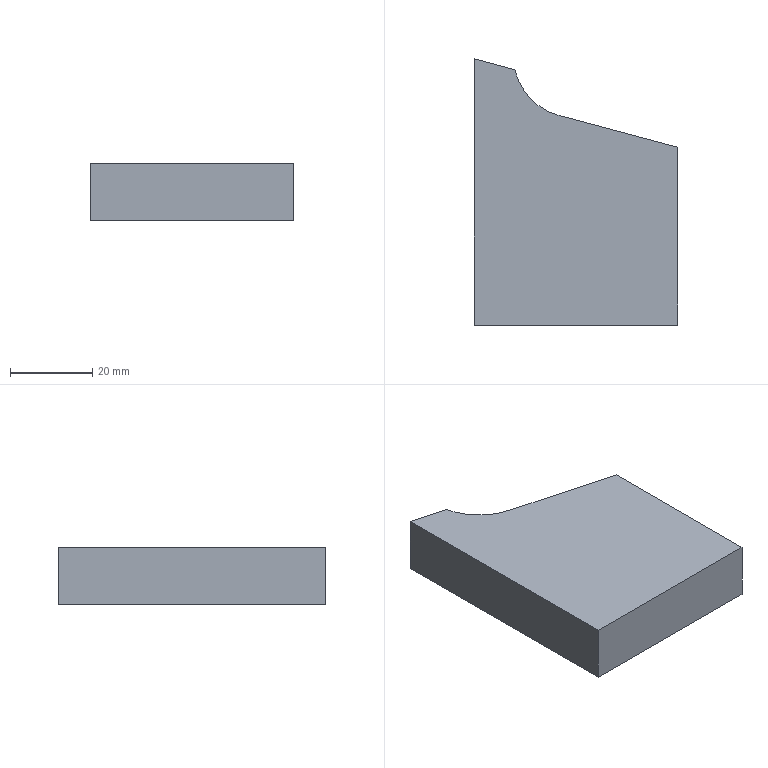Part | NX | features MOVE_FACE 3, pipe ejector 2 | 1 solid | 8 faces | box 49.5 x 64.866 x 14 mm | volume 36068 mm3 | plane 7 | cylinder 1 | commonest cylinder face diameters 30 x1
STEP:
#1=CARTESIAN_POINT('',(-49.5,13.263,-14.5));
#2=VERTEX_POINT('',#1);
#3=CARTESIAN_POINT('',(-49.5,-51.603,-14.5));
#4=VERTEX_POINT('',#3);
#5=CARTESIAN_POINT('',(-49.5,-51.603,-14.5));
#6=DIRECTION('',(0.,-1.,0.));
#7=VECTOR('',#6,1000.);
#8=LINE('',#5,#7);
#9=EDGE_CURVE('',#2,#4,#8,.T.);
#10=ORIENTED_EDGE('',*,*,#9,.F.);
#11=CARTESIAN_POINT('',(-39.626,10.618,-14.5));
#12=VERTEX_POINT('',#11);
#13=CARTESIAN_POINT('',(-50.,13.397,-14.5));
#14=DIRECTION('',(-0.9659,0.2588,0.));
#15=VECTOR('',#14,1000.);
#16=LINE('',#13,#15);
#17=EDGE_CURVE('',#12,#2,#16,.T.);
#18=ORIENTED_EDGE('',*,*,#17,.F.);
#19=CARTESIAN_POINT('',(-28.882,-0.5432,-14.5));
#20=VERTEX_POINT('',#19);
#21=CARTESIAN_POINT('',(-25.,13.946,-14.5));
#22=DIRECTION('',(0.,0.,1.));
#23=DIRECTION('',(1.,0.,0.));
#24=AXIS2_PLACEMENT_3D('',#21,#22,#23);
#25=CIRCLE('',#24,15.);
#26=EDGE_CURVE('',#12,#20,#25,.T.);
#27=ORIENTED_EDGE('',*,*,#26,.T.);
#28=CARTESIAN_POINT('',(0.,-8.282,-14.5));
#29=VERTEX_POINT('',#28);
#30=CARTESIAN_POINT('',(-28.882,-0.5432,-14.5));
#31=DIRECTION('',(0.9659,-0.2588,0.));
#32=VECTOR('',#31,1000.);
#33=LINE('',#30,#32);
#34=EDGE_CURVE('',#20,#29,#33,.T.);
#35=ORIENTED_EDGE('',*,*,#34,.T.);
#36=CARTESIAN_POINT('',(0.,-51.603,-14.5));
#37=VERTEX_POINT('',#36);
#38=CARTESIAN_POINT('',(0.,0.,-14.5));
#39=DIRECTION('',(0.,1.,0.));
#40=VECTOR('',#39,1000.);
#41=LINE('',#38,#40);
#42=EDGE_CURVE('',#37,#29,#41,.T.);
#43=ORIENTED_EDGE('',*,*,#42,.F.);
#44=CARTESIAN_POINT('',(0.,-51.603,-14.5));
#45=DIRECTION('',(1.,0.,0.));
#46=VECTOR('',#45,1000.);
#47=LINE('',#44,#46);
#48=EDGE_CURVE('',#4,#37,#47,.T.);
#49=ORIENTED_EDGE('',*,*,#48,.F.);
#50=EDGE_LOOP('',(#10,#18,#27,#35,#43,#49));
#51=FACE_BOUND('',#50,.T.);
#52=CARTESIAN_POINT('',(0.,0.,-14.5));
#53=DIRECTION('',(0.,0.,-1.));
#54=DIRECTION('',(-1.,0.,0.));
#55=AXIS2_PLACEMENT_3D('',#52,#53,#54);
#56=PLANE('',#55);
#57=ADVANCED_FACE('',(#51),#56,.T.);
#58=CARTESIAN_POINT('',(0.,-51.603,-0.5));
#59=VERTEX_POINT('',#58);
#60=CARTESIAN_POINT('',(0.,-51.603,-15.));
#61=DIRECTION('',(0.,0.,1.));
#62=VECTOR('',#61,1000.);
#63=LINE('',#60,#62);
#64=EDGE_CURVE('',#37,#59,#63,.T.);
#65=ORIENTED_EDGE('',*,*,#64,.F.);
#66=ORIENTED_EDGE('',*,*,#42,.T.);
#67=CARTESIAN_POINT('',(0.,-8.282,-0.5));
#68=VERTEX_POINT('',#67);
#69=CARTESIAN_POINT('',(0.,-8.282,-15.));
#70=DIRECTION('',(0.,0.,1.));
#71=VECTOR('',#70,1000.);
#72=LINE('',#69,#71);
#73=EDGE_CURVE('',#29,#68,#72,.T.);
#74=ORIENTED_EDGE('',*,*,#73,.T.);
#75=CARTESIAN_POINT('',(0.,0.,-0.5));
#76=DIRECTION('',(0.,1.,0.));
#77=VECTOR('',#76,1000.);
#78=LINE('',#75,#77);
#79=EDGE_CURVE('',#68,#59,#78,.F.);
#80=ORIENTED_EDGE('',*,*,#79,.T.);
#81=EDGE_LOOP('',(#65,#66,#74,#80));
#82=FACE_BOUND('',#81,.T.);
#83=CARTESIAN_POINT('',(0.,0.,-15.));
#84=DIRECTION('',(1.,0.,0.));
#85=DIRECTION('',(0.,1.,0.));
#86=AXIS2_PLACEMENT_3D('',#83,#84,#85);
#87=PLANE('',#86);
#88=ADVANCED_FACE('',(#82),#87,.T.);
#89=ORIENTED_EDGE('',*,*,#48,.T.);
#90=ORIENTED_EDGE('',*,*,#64,.T.);
#91=CARTESIAN_POINT('',(-49.5,-51.603,-0.5));
#92=VERTEX_POINT('',#91);
#93=CARTESIAN_POINT('',(0.,-51.603,-0.5));
#94=DIRECTION('',(-1.,0.,0.));
#95=VECTOR('',#94,1000.);
#96=LINE('',#93,#95);
#97=EDGE_CURVE('',#59,#92,#96,.T.);
#98=ORIENTED_EDGE('',*,*,#97,.T.);
#99=CARTESIAN_POINT('',(-49.5,-51.603,-15.));
#100=DIRECTION('',(0.,0.,1.));
#101=VECTOR('',#100,1000.);
#102=LINE('',#99,#101);
#103=EDGE_CURVE('',#4,#92,#102,.T.);
#104=ORIENTED_EDGE('',*,*,#103,.F.);
#105=EDGE_LOOP('',(#89,#90,#98,#104));
#106=FACE_BOUND('',#105,.T.);
#107=CARTESIAN_POINT('',(0.,-51.603,-15.));
#108=DIRECTION('',(0.,-1.,0.));
#109=DIRECTION('',(1.,0.,0.));
#110=AXIS2_PLACEMENT_3D('',#107,#108,#109);
#111=PLANE('',#110);
#112=ADVANCED_FACE('',(#106),#111,.T.);
#113=ORIENTED_EDGE('',*,*,#9,.T.);
#114=ORIENTED_EDGE('',*,*,#103,.T.);
#115=CARTESIAN_POINT('',(-49.5,13.263,-0.5));
#116=VERTEX_POINT('',#115);
#117=CARTESIAN_POINT('',(-49.5,0.,-0.5));
#118=DIRECTION('',(0.,1.,0.));
#119=VECTOR('',#118,1000.);
#120=LINE('',#117,#119);
#121=EDGE_CURVE('',#92,#116,#120,.T.);
#122=ORIENTED_EDGE('',*,*,#121,.T.);
#123=CARTESIAN_POINT('',(-49.5,13.263,-15.));
#124=DIRECTION('',(0.,0.,1.));
#125=VECTOR('',#124,1000.);
#126=LINE('',#123,#125);
#127=EDGE_CURVE('',#2,#116,#126,.T.);
#128=ORIENTED_EDGE('',*,*,#127,.F.);
#129=EDGE_LOOP('',(#113,#114,#122,#128));
#130=FACE_BOUND('',#129,.T.);
#131=CARTESIAN_POINT('',(-49.5,-51.603,-15.));
#132=DIRECTION('',(-1.,0.,0.));
#133=DIRECTION('',(0.,-1.,0.));
#134=AXIS2_PLACEMENT_3D('',#131,#132,#133);
#135=PLANE('',#134);
#136=ADVANCED_FACE('',(#130),#135,.T.);
#137=ORIENTED_EDGE('',*,*,#127,.T.);
#138=CARTESIAN_POINT('',(-39.626,10.618,-0.5));
#139=VERTEX_POINT('',#138);
#140=CARTESIAN_POINT('',(-50.,13.397,-0.5));
#141=DIRECTION('',(0.9659,-0.2588,0.));
#142=VECTOR('',#141,1000.);
#143=LINE('',#140,#142);
#144=EDGE_CURVE('',#116,#139,#143,.T.);
#145=ORIENTED_EDGE('',*,*,#144,.T.);
#146=CARTESIAN_POINT('',(-39.626,10.618,-15.));
#147=DIRECTION('',(0.,0.,1.));
#148=VECTOR('',#147,1000.);
#149=LINE('',#146,#148);
#150=EDGE_CURVE('',#139,#12,#149,.F.);
#151=ORIENTED_EDGE('',*,*,#150,.T.);
#152=ORIENTED_EDGE('',*,*,#17,.T.);
#153=EDGE_LOOP('',(#137,#145,#151,#152));
#154=FACE_BOUND('',#153,.T.);
#155=CARTESIAN_POINT('',(-50.,13.397,-15.));
#156=DIRECTION('',(0.2588,0.9659,0.));
#157=DIRECTION('',(-0.9659,0.2588,0.));
#158=AXIS2_PLACEMENT_3D('',#155,#156,#157);
#159=PLANE('',#158);
#160=ADVANCED_FACE('',(#154),#159,.T.);
#161=CARTESIAN_POINT('',(-28.882,-0.5432,-0.5));
#162=VERTEX_POINT('',#161);
#163=CARTESIAN_POINT('',(-25.,13.946,-0.5));
#164=DIRECTION('',(0.,0.,1.));
#165=DIRECTION('',(1.,0.,0.));
#166=AXIS2_PLACEMENT_3D('',#163,#164,#165);
#167=CIRCLE('',#166,15.);
#168=EDGE_CURVE('',#139,#162,#167,.T.);
#169=ORIENTED_EDGE('',*,*,#168,.T.);
#170=CARTESIAN_POINT('',(-28.882,-0.5432,-15.));
#171=DIRECTION('',(0.,0.,1.));
#172=VECTOR('',#171,1000.);
#173=LINE('',#170,#172);
#174=EDGE_CURVE('',#162,#20,#173,.F.);
#175=ORIENTED_EDGE('',*,*,#174,.T.);
#176=ORIENTED_EDGE('',*,*,#26,.F.);
#177=ORIENTED_EDGE('',*,*,#150,.F.);
#178=EDGE_LOOP('',(#169,#175,#176,#177));
#179=FACE_BOUND('',#178,.T.);
#180=CARTESIAN_POINT('',(-25.,13.946,-15.));
#181=DIRECTION('',(0.,0.,1.));
#182=DIRECTION('',(1.,0.,0.));
#183=AXIS2_PLACEMENT_3D('',#180,#181,#182);
#184=CYLINDRICAL_SURFACE('',#183,15.);
#185=ADVANCED_FACE('',(#179),#184,.F.);
#186=ORIENTED_EDGE('',*,*,#34,.F.);
#187=ORIENTED_EDGE('',*,*,#174,.F.);
#188=CARTESIAN_POINT('',(-28.882,-0.5432,-0.5));
#189=DIRECTION('',(0.9659,-0.2588,0.));
#190=VECTOR('',#189,1000.);
#191=LINE('',#188,#190);
#192=EDGE_CURVE('',#162,#68,#191,.T.);
#193=ORIENTED_EDGE('',*,*,#192,.T.);
#194=ORIENTED_EDGE('',*,*,#73,.F.);
#195=EDGE_LOOP('',(#186,#187,#193,#194));
#196=FACE_BOUND('',#195,.T.);
#197=CARTESIAN_POINT('',(-28.882,-0.5432,-15.));
#198=DIRECTION('',(-0.2588,-0.9659,0.));
#199=DIRECTION('',(0.9659,-0.2588,0.));
#200=AXIS2_PLACEMENT_3D('',#197,#198,#199);
#201=PLANE('',#200);
#202=ADVANCED_FACE('',(#196),#201,.F.);
#203=ORIENTED_EDGE('',*,*,#168,.F.);
#204=ORIENTED_EDGE('',*,*,#144,.F.);
#205=ORIENTED_EDGE('',*,*,#121,.F.);
#206=ORIENTED_EDGE('',*,*,#97,.F.);
#207=ORIENTED_EDGE('',*,*,#79,.F.);
#208=ORIENTED_EDGE('',*,*,#192,.F.);
#209=EDGE_LOOP('',(#203,#204,#205,#206,#207,#208));
#210=FACE_BOUND('',#209,.T.);
#211=CARTESIAN_POINT('',(0.,0.,-0.5));
#212=DIRECTION('',(0.,0.,-1.));
#213=DIRECTION('',(-1.,0.,0.));
#214=AXIS2_PLACEMENT_3D('',#211,#212,#213);
#215=PLANE('',#214);
#216=ADVANCED_FACE('',(#210),#215,.F.);
#217=CLOSED_SHELL('',(#57,#88,#112,#136,#160,#185,#202,#216));
#218=MANIFOLD_SOLID_BREP('',#217);
#219=(LENGTH_UNIT()NAMED_UNIT(*)SI_UNIT(.MILLI.,.METRE.));
#220=UNCERTAINTY_MEASURE_WITH_UNIT(LENGTH_MEASURE(0.00001),#219,'','');
#221=(NAMED_UNIT(*)PLANE_ANGLE_UNIT()SI_UNIT($,.RADIAN.));
#222=(NAMED_UNIT(*)SI_UNIT($,.STERADIAN.)SOLID_ANGLE_UNIT());
#223=(GEOMETRIC_REPRESENTATION_CONTEXT(3)GLOBAL_UNCERTAINTY_ASSIGNED_CONTEXT((#220))GLOBAL_UNIT_ASSIGNED_CONTEXT((#219,#221,#222))REPRESENTATION_CONTEXT('',''));
#224=ADVANCED_BREP_SHAPE_REPRESENTATION('',(#218),#223);